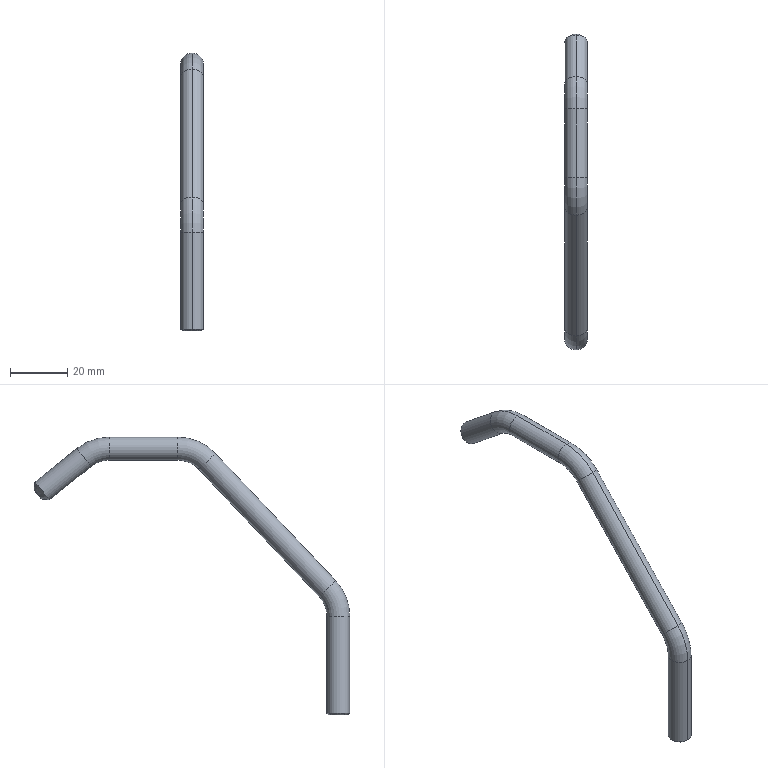Part | STEP file | 8XS234010 | 1 solid | 20 faces | box 8 x 110.249 x 97 mm | volume 8595 mm3 | cylinder 8 | torus 6 | cone 4 | plane 2 | commonest cylinder face diameters 8 x8
STEP:
#1=CARTESIAN_POINT('',(0.,0.,0.));
#2=DIRECTION('',(0.,0.,1.));
#3=DIRECTION('',(1.,0.,0.));
#4=AXIS2_PLACEMENT_3D('',#1,#2,#3);
#5=CARTESIAN_POINT('',(0.,4.,34.438));
#6=VERTEX_POINT('',#5);
#7=CARTESIAN_POINT('',(0.,-4.,34.438));
#8=VERTEX_POINT('',#7);
#9=CARTESIAN_POINT('',(0.,0.,34.438));
#10=DIRECTION('',(0.,0.,1.));
#11=DIRECTION('',(1.,0.,0.));
#12=AXIS2_PLACEMENT_3D('',#9,#10,#11);
#13=CIRCLE('',#12,4.);
#14=CARTESIAN_POINT('',(0.,14.,34.438));
#15=DIRECTION('',(-1.,0.,0.));
#16=DIRECTION('',(0.,0.,1.));
#17=AXIS2_PLACEMENT_3D('',#14,#15,#16);
#18=TOROIDAL_SURFACE('',#17,14.,4.);
#19=CARTESIAN_POINT('',(4.712,4.712));
#20=DIRECTION('',(0.,-1.));
#21=VECTOR('',#20,1.);
#22=LINE('',#19,#21);
#23=(GEOMETRIC_REPRESENTATION_CONTEXT(2)PARAMETRIC_REPRESENTATION_CONTEXT()REPRESENTATION_CONTEXT('',''));
#24=DEFINITIONAL_REPRESENTATION('',(#22),#23);
#25=PCURVE('',#18,#24);
#26=CARTESIAN_POINT('',(0.,0.,34.438));
#27=DIRECTION('',(0.,0.,-1.));
#28=DIRECTION('',(0.,1.,0.));
#29=AXIS2_PLACEMENT_3D('',#26,#27,#28);
#30=CYLINDRICAL_SURFACE('',#29,4.);
#31=CARTESIAN_POINT('',(7.854,0.));
#32=DIRECTION('',(-1.,0.));
#33=VECTOR('',#32,1.);
#34=LINE('',#31,#33);
#35=(GEOMETRIC_REPRESENTATION_CONTEXT(2)PARAMETRIC_REPRESENTATION_CONTEXT()REPRESENTATION_CONTEXT('',''));
#36=DEFINITIONAL_REPRESENTATION('',(#34),#35);
#37=PCURVE('',#30,#36);
#38=SURFACE_CURVE('',#13,(#25,#37),.PCURVE_S1.);
#39=EDGE_CURVE('',#6,#8,#38,.T.);
#40=ORIENTED_EDGE('',*,*,#39,.T.);
#41=CARTESIAN_POINT('',(0.,0.9069,46.79));
#42=VERTEX_POINT('',#41);
#43=CARTESIAN_POINT('',(0.,14.,34.438));
#44=DIRECTION('',(-1.,0.,0.));
#45=DIRECTION('',(0.,0.,1.));
#46=AXIS2_PLACEMENT_3D('',#43,#44,#45);
#47=CIRCLE('',#46,18.);
#48=CARTESIAN_POINT('',(0.,0.));
#49=DIRECTION('',(1.,0.));
#50=VECTOR('',#49,1.);
#51=LINE('',#48,#50);
#52=(GEOMETRIC_REPRESENTATION_CONTEXT(2)PARAMETRIC_REPRESENTATION_CONTEXT()REPRESENTATION_CONTEXT('',''));
#53=DEFINITIONAL_REPRESENTATION('',(#51),#52);
#54=PCURVE('',#18,#53);
#55=CARTESIAN_POINT('',(0.,14.,34.438));
#56=DIRECTION('',(-1.,0.,0.));
#57=DIRECTION('',(0.,0.,1.));
#58=AXIS2_PLACEMENT_3D('',#55,#56,#57);
#59=TOROIDAL_SURFACE('',#58,14.,4.);
#60=CARTESIAN_POINT('',(0.,6.283));
#61=DIRECTION('',(1.,0.));
#62=VECTOR('',#61,1.);
#63=LINE('',#60,#62);
#64=(GEOMETRIC_REPRESENTATION_CONTEXT(2)PARAMETRIC_REPRESENTATION_CONTEXT()REPRESENTATION_CONTEXT('',''));
#65=DEFINITIONAL_REPRESENTATION('',(#63),#64);
#66=PCURVE('',#59,#65);
#67=SURFACE_CURVE('',#47,(#54,#66),.PCURVE_S1.);
#68=EDGE_CURVE('',#8,#42,#67,.T.);
#69=ORIENTED_EDGE('',*,*,#68,.T.);
#70=CARTESIAN_POINT('',(0.,6.726,41.301));
#71=VERTEX_POINT('',#70);
#72=CARTESIAN_POINT('',(0.,3.816,44.045));
#73=DIRECTION('',(0.,0.6862,0.7274));
#74=DIRECTION('',(1.,0.,0.));
#75=AXIS2_PLACEMENT_3D('',#72,#73,#74);
#76=CIRCLE('',#75,4.);
#77=CARTESIAN_POINT('',(5.469,4.712));
#78=DIRECTION('',(0.,-1.));
#79=VECTOR('',#78,1.);
#80=LINE('',#77,#79);
#81=(GEOMETRIC_REPRESENTATION_CONTEXT(2)PARAMETRIC_REPRESENTATION_CONTEXT()REPRESENTATION_CONTEXT('',''));
#82=DEFINITIONAL_REPRESENTATION('',(#80),#81);
#83=PCURVE('',#18,#82);
#84=CARTESIAN_POINT('',(0.,3.816,44.045));
#85=DIRECTION('',(0.,0.6862,0.7274));
#86=DIRECTION('',(0.,-0.7274,0.6862));
#87=AXIS2_PLACEMENT_3D('',#84,#85,#86);
#88=CYLINDRICAL_SURFACE('',#87,4.);
#89=CARTESIAN_POINT('',(1.571,0.));
#90=DIRECTION('',(1.,0.));
#91=VECTOR('',#90,1.);
#92=LINE('',#89,#91);
#93=(GEOMETRIC_REPRESENTATION_CONTEXT(2)PARAMETRIC_REPRESENTATION_CONTEXT()REPRESENTATION_CONTEXT('',''));
#94=DEFINITIONAL_REPRESENTATION('',(#92),#93);
#95=PCURVE('',#88,#94);
#96=SURFACE_CURVE('',#76,(#83,#95),.PCURVE_S1.);
#97=EDGE_CURVE('',#71,#42,#96,.T.);
#98=ORIENTED_EDGE('',*,*,#97,.F.);
#99=CARTESIAN_POINT('',(0.,14.,34.438));
#100=DIRECTION('',(-1.,0.,0.));
#101=DIRECTION('',(0.,0.,1.));
#102=AXIS2_PLACEMENT_3D('',#99,#100,#101);
#103=CIRCLE('',#102,10.);
#104=CARTESIAN_POINT('',(0.,3.142));
#105=DIRECTION('',(1.,0.));
#106=VECTOR('',#105,1.);
#107=LINE('',#104,#106);
#108=(GEOMETRIC_REPRESENTATION_CONTEXT(2)PARAMETRIC_REPRESENTATION_CONTEXT()REPRESENTATION_CONTEXT('',''));
#109=DEFINITIONAL_REPRESENTATION('',(#107),#108);
#110=PCURVE('',#18,#109);
#111=CARTESIAN_POINT('',(0.,3.142));
#112=DIRECTION('',(1.,0.));
#113=VECTOR('',#112,1.);
#114=LINE('',#111,#113);
#115=(GEOMETRIC_REPRESENTATION_CONTEXT(2)PARAMETRIC_REPRESENTATION_CONTEXT()REPRESENTATION_CONTEXT('',''));
#116=DEFINITIONAL_REPRESENTATION('',(#114),#115);
#117=PCURVE('',#59,#116);
#118=SURFACE_CURVE('',#103,(#110,#117),.PCURVE_S1.);
#119=EDGE_CURVE('',#6,#71,#118,.T.);
#120=ORIENTED_EDGE('',*,*,#119,.F.);
#121=EDGE_LOOP('',(#40,#69,#98,#120));
#122=FACE_BOUND('',#121,.T.);
#123=ADVANCED_FACE('',(#122),#18,.T.);
#124=CARTESIAN_POINT('',(0.,48.765,85.862));
#125=VERTEX_POINT('',#124);
#126=CARTESIAN_POINT('',(0.,42.946,91.352));
#127=VERTEX_POINT('',#126);
#128=CARTESIAN_POINT('',(0.,45.856,88.607));
#129=DIRECTION('',(0.,0.6862,0.7274));
#130=DIRECTION('',(1.,0.,0.));
#131=AXIS2_PLACEMENT_3D('',#128,#129,#130);
#132=CIRCLE('',#131,4.);
#133=CARTESIAN_POINT('',(0.,56.039,79.));
#134=DIRECTION('',(-1.,0.,0.));
#135=DIRECTION('',(0.,0.,1.));
#136=AXIS2_PLACEMENT_3D('',#133,#134,#135);
#137=TOROIDAL_SURFACE('',#136,14.,4.);
#138=CARTESIAN_POINT('',(5.469,4.712));
#139=DIRECTION('',(0.,-1.));
#140=VECTOR('',#139,1.);
#141=LINE('',#138,#140);
#142=(GEOMETRIC_REPRESENTATION_CONTEXT(2)PARAMETRIC_REPRESENTATION_CONTEXT()REPRESENTATION_CONTEXT('',''));
#143=DEFINITIONAL_REPRESENTATION('',(#141),#142);
#144=PCURVE('',#137,#143);
#145=CARTESIAN_POINT('',(1.571,61.262));
#146=DIRECTION('',(1.,0.));
#147=VECTOR('',#146,1.);
#148=LINE('',#145,#147);
#149=(GEOMETRIC_REPRESENTATION_CONTEXT(2)PARAMETRIC_REPRESENTATION_CONTEXT()REPRESENTATION_CONTEXT('',''));
#150=DEFINITIONAL_REPRESENTATION('',(#148),#149);
#151=PCURVE('',#88,#150);
#152=SURFACE_CURVE('',#132,(#144,#151),.PCURVE_S1.);
#153=EDGE_CURVE('',#125,#127,#152,.T.);
#154=ORIENTED_EDGE('',*,*,#153,.T.);
#155=CARTESIAN_POINT('',(0.,56.039,97.));
#156=VERTEX_POINT('',#155);
#157=CARTESIAN_POINT('',(0.,56.039,79.));
#158=DIRECTION('',(-1.,0.,0.));
#159=DIRECTION('',(0.,0.,1.));
#160=AXIS2_PLACEMENT_3D('',#157,#158,#159);
#161=CIRCLE('',#160,18.);
#162=CARTESIAN_POINT('',(0.,0.));
#163=DIRECTION('',(1.,0.));
#164=VECTOR('',#163,1.);
#165=LINE('',#162,#164);
#166=(GEOMETRIC_REPRESENTATION_CONTEXT(2)PARAMETRIC_REPRESENTATION_CONTEXT()REPRESENTATION_CONTEXT('',''));
#167=DEFINITIONAL_REPRESENTATION('',(#165),#166);
#168=PCURVE('',#137,#167);
#169=CARTESIAN_POINT('',(0.,56.039,79.));
#170=DIRECTION('',(-1.,0.,0.));
#171=DIRECTION('',(0.,0.,1.));
#172=AXIS2_PLACEMENT_3D('',#169,#170,#171);
#173=TOROIDAL_SURFACE('',#172,14.,4.);
#174=CARTESIAN_POINT('',(0.,6.283));
#175=DIRECTION('',(1.,0.));
#176=VECTOR('',#175,1.);
#177=LINE('',#174,#176);
#178=(GEOMETRIC_REPRESENTATION_CONTEXT(2)PARAMETRIC_REPRESENTATION_CONTEXT()REPRESENTATION_CONTEXT('',''));
#179=DEFINITIONAL_REPRESENTATION('',(#177),#178);
#180=PCURVE('',#173,#179);
#181=SURFACE_CURVE('',#161,(#168,#180),.PCURVE_S1.);
#182=EDGE_CURVE('',#127,#156,#181,.T.);
#183=ORIENTED_EDGE('',*,*,#182,.T.);
#184=CARTESIAN_POINT('',(0.,56.039,89.));
#185=VERTEX_POINT('',#184);
#186=CARTESIAN_POINT('',(0.,56.039,93.));
#187=DIRECTION('',(0.,1.,0.));
#188=DIRECTION('',(1.,0.,0.));
#189=AXIS2_PLACEMENT_3D('',#186,#187,#188);
#190=CIRCLE('',#189,4.);
#191=CARTESIAN_POINT('',(6.283,4.712));
#192=DIRECTION('',(0.,-1.));
#193=VECTOR('',#192,1.);
#194=LINE('',#191,#193);
#195=(GEOMETRIC_REPRESENTATION_CONTEXT(2)PARAMETRIC_REPRESENTATION_CONTEXT()REPRESENTATION_CONTEXT('',''));
#196=DEFINITIONAL_REPRESENTATION('',(#194),#195);
#197=PCURVE('',#137,#196);
#198=CARTESIAN_POINT('',(0.,56.039,93.));
#199=DIRECTION('',(0.,1.,0.));
#200=DIRECTION('',(0.,0.,1.));
#201=AXIS2_PLACEMENT_3D('',#198,#199,#200);
#202=CYLINDRICAL_SURFACE('',#201,4.);
#203=CARTESIAN_POINT('',(1.571,0.));
#204=DIRECTION('',(1.,0.));
#205=VECTOR('',#204,1.);
#206=LINE('',#203,#205);
#207=(GEOMETRIC_REPRESENTATION_CONTEXT(2)PARAMETRIC_REPRESENTATION_CONTEXT()REPRESENTATION_CONTEXT('',''));
#208=DEFINITIONAL_REPRESENTATION('',(#206),#207);
#209=PCURVE('',#202,#208);
#210=SURFACE_CURVE('',#190,(#197,#209),.PCURVE_S1.);
#211=EDGE_CURVE('',#185,#156,#210,.T.);
#212=ORIENTED_EDGE('',*,*,#211,.F.);
#213=CARTESIAN_POINT('',(0.,56.039,79.));
#214=DIRECTION('',(-1.,0.,0.));
#215=DIRECTION('',(0.,0.,1.));
#216=AXIS2_PLACEMENT_3D('',#213,#214,#215);
#217=CIRCLE('',#216,10.);
#218=CARTESIAN_POINT('',(0.,3.142));
#219=DIRECTION('',(1.,0.));
#220=VECTOR('',#219,1.);
#221=LINE('',#218,#220);
#222=(GEOMETRIC_REPRESENTATION_CONTEXT(2)PARAMETRIC_REPRESENTATION_CONTEXT()REPRESENTATION_CONTEXT('',''));
#223=DEFINITIONAL_REPRESENTATION('',(#221),#222);
#224=PCURVE('',#137,#223);
#225=CARTESIAN_POINT('',(0.,3.142));
#226=DIRECTION('',(1.,0.));
#227=VECTOR('',#226,1.);
#228=LINE('',#225,#227);
#229=(GEOMETRIC_REPRESENTATION_CONTEXT(2)PARAMETRIC_REPRESENTATION_CONTEXT()REPRESENTATION_CONTEXT('',''));
#230=DEFINITIONAL_REPRESENTATION('',(#228),#229);
#231=PCURVE('',#173,#230);
#232=SURFACE_CURVE('',#217,(#224,#231),.PCURVE_S1.);
#233=EDGE_CURVE('',#125,#185,#232,.T.);
#234=ORIENTED_EDGE('',*,*,#233,.F.);
#235=EDGE_LOOP('',(#154,#183,#212,#234));
#236=FACE_BOUND('',#235,.T.);
#237=ADVANCED_FACE('',(#236),#137,.T.);
#238=CARTESIAN_POINT('',(0.,80.089,89.));
#239=VERTEX_POINT('',#238);
#240=CARTESIAN_POINT('',(0.,80.089,97.));
#241=VERTEX_POINT('',#240);
#242=CARTESIAN_POINT('',(0.,80.089,93.));
#243=DIRECTION('',(0.,1.,0.));
#244=DIRECTION('',(1.,0.,0.));
#245=AXIS2_PLACEMENT_3D('',#242,#243,#244);
#246=CIRCLE('',#245,4.);
#247=CARTESIAN_POINT('',(0.,80.089,79.));
#248=DIRECTION('',(-1.,0.,0.));
#249=DIRECTION('',(0.,0.,1.));
#250=AXIS2_PLACEMENT_3D('',#247,#248,#249);
#251=TOROIDAL_SURFACE('',#250,14.,4.);
#252=CARTESIAN_POINT('',(0.,4.712));
#253=DIRECTION('',(0.,-1.));
#254=VECTOR('',#253,1.);
#255=LINE('',#252,#254);
#256=(GEOMETRIC_REPRESENTATION_CONTEXT(2)PARAMETRIC_REPRESENTATION_CONTEXT()REPRESENTATION_CONTEXT('',''));
#257=DEFINITIONAL_REPRESENTATION('',(#255),#256);
#258=PCURVE('',#251,#257);
#259=CARTESIAN_POINT('',(1.571,24.05));
#260=DIRECTION('',(1.,0.));
#261=VECTOR('',#260,1.);
#262=LINE('',#259,#261);
#263=(GEOMETRIC_REPRESENTATION_CONTEXT(2)PARAMETRIC_REPRESENTATION_CONTEXT()REPRESENTATION_CONTEXT('',''));
#264=DEFINITIONAL_REPRESENTATION('',(#262),#263);
#265=PCURVE('',#202,#264);
#266=SURFACE_CURVE('',#246,(#258,#265),.PCURVE_S1.);
#267=EDGE_CURVE('',#239,#241,#266,.T.);
#268=ORIENTED_EDGE('',*,*,#267,.T.);
#269=CARTESIAN_POINT('',(0.,91.334,93.056));
#270=VERTEX_POINT('',#269);
#271=CARTESIAN_POINT('',(0.,80.089,79.));
#272=DIRECTION('',(-1.,0.,0.));
#273=DIRECTION('',(0.,0.,1.));
#274=AXIS2_PLACEMENT_3D('',#271,#272,#273);
#275=CIRCLE('',#274,18.);
#276=CARTESIAN_POINT('',(0.,0.));
#277=DIRECTION('',(1.,0.));
#278=VECTOR('',#277,1.);
#279=LINE('',#276,#278);
#280=(GEOMETRIC_REPRESENTATION_CONTEXT(2)PARAMETRIC_REPRESENTATION_CONTEXT()REPRESENTATION_CONTEXT('',''));
#281=DEFINITIONAL_REPRESENTATION('',(#279),#280);
#282=PCURVE('',#251,#281);
#283=CARTESIAN_POINT('',(0.,80.089,79.));
#284=DIRECTION('',(-1.,0.,0.));
#285=DIRECTION('',(0.,0.,1.));
#286=AXIS2_PLACEMENT_3D('',#283,#284,#285);
#287=TOROIDAL_SURFACE('',#286,14.,4.);
#288=CARTESIAN_POINT('',(0.,6.283));
#289=DIRECTION('',(1.,0.));
#290=VECTOR('',#289,1.);
#291=LINE('',#288,#290);
#292=(GEOMETRIC_REPRESENTATION_CONTEXT(2)PARAMETRIC_REPRESENTATION_CONTEXT()REPRESENTATION_CONTEXT('',''));
#293=DEFINITIONAL_REPRESENTATION('',(#291),#292);
#294=PCURVE('',#287,#293);
#295=SURFACE_CURVE('',#275,(#282,#294),.PCURVE_S1.);
#296=EDGE_CURVE('',#241,#270,#295,.T.);
#297=ORIENTED_EDGE('',*,*,#296,.T.);
#298=CARTESIAN_POINT('',(0.,86.336,86.809));
#299=VERTEX_POINT('',#298);
#300=CARTESIAN_POINT('',(0.,88.835,89.932));
#301=DIRECTION('',(0.,0.7809,-0.6247));
#302=DIRECTION('',(1.,0.,0.));
#303=AXIS2_PLACEMENT_3D('',#300,#301,#302);
#304=CIRCLE('',#303,4.);
#305=CARTESIAN_POINT('',(0.6747,4.712));
#306=DIRECTION('',(0.,-1.));
#307=VECTOR('',#306,1.);
#308=LINE('',#305,#307);
#309=(GEOMETRIC_REPRESENTATION_CONTEXT(2)PARAMETRIC_REPRESENTATION_CONTEXT()REPRESENTATION_CONTEXT('',''));
#310=DEFINITIONAL_REPRESENTATION('',(#308),#309);
#311=PCURVE('',#251,#310);
#312=CARTESIAN_POINT('',(0.,88.835,89.932));
#313=DIRECTION('',(0.,0.7809,-0.6247));
#314=DIRECTION('',(0.,0.6247,0.7809));
#315=AXIS2_PLACEMENT_3D('',#312,#313,#314);
#316=CYLINDRICAL_SURFACE('',#315,4.);
#317=CARTESIAN_POINT('',(1.571,0.));
#318=DIRECTION('',(1.,0.));
#319=VECTOR('',#318,1.);
#320=LINE('',#317,#319);
#321=(GEOMETRIC_REPRESENTATION_CONTEXT(2)PARAMETRIC_REPRESENTATION_CONTEXT()REPRESENTATION_CONTEXT('',''));
#322=DEFINITIONAL_REPRESENTATION('',(#320),#321);
#323=PCURVE('',#316,#322);
#324=SURFACE_CURVE('',#304,(#311,#323),.PCURVE_S1.);
#325=EDGE_CURVE('',#299,#270,#324,.T.);
#326=ORIENTED_EDGE('',*,*,#325,.F.);
#327=CARTESIAN_POINT('',(0.,80.089,79.));
#328=DIRECTION('',(-1.,0.,0.));
#329=DIRECTION('',(0.,0.,1.));
#330=AXIS2_PLACEMENT_3D('',#327,#328,#329);
#331=CIRCLE('',#330,10.);
#332=CARTESIAN_POINT('',(0.,3.142));
#333=DIRECTION('',(1.,0.));
#334=VECTOR('',#333,1.);
#335=LINE('',#332,#334);
#336=(GEOMETRIC_REPRESENTATION_CONTEXT(2)PARAMETRIC_REPRESENTATION_CONTEXT()REPRESENTATION_CONTEXT('',''));
#337=DEFINITIONAL_REPRESENTATION('',(#335),#336);
#338=PCURVE('',#251,#337);
#339=CARTESIAN_POINT('',(0.,3.142));
#340=DIRECTION('',(1.,0.));
#341=VECTOR('',#340,1.);
#342=LINE('',#339,#341);
#343=(GEOMETRIC_REPRESENTATION_CONTEXT(2)PARAMETRIC_REPRESENTATION_CONTEXT()REPRESENTATION_CONTEXT('',''));
#344=DEFINITIONAL_REPRESENTATION('',(#342),#343);
#345=PCURVE('',#287,#344);
#346=SURFACE_CURVE('',#331,(#338,#345),.PCURVE_S1.);
#347=EDGE_CURVE('',#239,#299,#346,.T.);
#348=ORIENTED_EDGE('',*,*,#347,.F.);
#349=EDGE_LOOP('',(#268,#297,#326,#348));
#350=FACE_BOUND('',#349,.T.);
#351=ADVANCED_FACE('',(#350),#251,.T.);
#352=CARTESIAN_POINT('',(0.,106.249,78.562));
#353=VERTEX_POINT('',#352);
#354=CARTESIAN_POINT('',(0.,103.751,75.438));
#355=VERTEX_POINT('',#354);
#356=CARTESIAN_POINT('',(0.,105.,77.));
#357=DIRECTION('',(0.,0.7809,-0.6247));
#358=DIRECTION('',(0.,0.6247,0.7809));
#359=AXIS2_PLACEMENT_3D('',#356,#357,#358);
#360=CIRCLE('',#359,2.);
#361=CARTESIAN_POINT('',(0.,105.,77.));
#362=DIRECTION('',(0.,-0.7809,0.6247));
#363=DIRECTION('',(0.,-0.6247,-0.7809));
#364=AXIS2_PLACEMENT_3D('',#361,#362,#363);
#365=CONICAL_SURFACE('',#364,2.,0.7854);
#366=CARTESIAN_POINT('',(3.142,0.));
#367=DIRECTION('',(-1.,0.));
#368=VECTOR('',#367,1.);
#369=LINE('',#366,#368);
#370=(GEOMETRIC_REPRESENTATION_CONTEXT(2)PARAMETRIC_REPRESENTATION_CONTEXT()REPRESENTATION_CONTEXT('',''));
#371=DEFINITIONAL_REPRESENTATION('',(#369),#370);
#372=PCURVE('',#365,#371);
#373=CARTESIAN_POINT('',(0.,105.,77.));
#374=DIRECTION('',(0.,0.7809,-0.6247));
#375=DIRECTION('',(1.,0.,0.));
#376=AXIS2_PLACEMENT_3D('',#373,#374,#375);
#377=PLANE('',#376);
#378=CARTESIAN_POINT('',(0.,0.));
#379=DIRECTION('',(0.,-1.));
#380=AXIS2_PLACEMENT_2D('',#378,#379);
#381=CIRCLE('',#380,2.);
#382=(GEOMETRIC_REPRESENTATION_CONTEXT(2)PARAMETRIC_REPRESENTATION_CONTEXT()REPRESENTATION_CONTEXT('',''));
#383=DEFINITIONAL_REPRESENTATION('',(#381),#382);
#384=PCURVE('',#377,#383);
#385=SURFACE_CURVE('',#360,(#372,#384),.PCURVE_S1.);
#386=EDGE_CURVE('',#353,#355,#385,.T.);
#387=ORIENTED_EDGE('',*,*,#386,.F.);
#388=CARTESIAN_POINT('',(0.,105.937,81.373));
#389=VERTEX_POINT('',#388);
#390=CARTESIAN_POINT('',(0.,106.249,78.562));
#391=DIRECTION('',(0.,-0.1104,0.9939));
#392=VECTOR('',#391,1.);
#393=LINE('',#390,#392);
#394=CARTESIAN_POINT('',(3.142,0.));
#395=DIRECTION('',(0.,1.));
#396=VECTOR('',#395,1.);
#397=LINE('',#394,#396);
#398=(GEOMETRIC_REPRESENTATION_CONTEXT(2)PARAMETRIC_REPRESENTATION_CONTEXT()REPRESENTATION_CONTEXT('',''));
#399=DEFINITIONAL_REPRESENTATION('',(#397),#398);
#400=PCURVE('',#365,#399);
#401=CARTESIAN_POINT('',(0.,105.,77.));
#402=DIRECTION('',(0.,-0.7809,0.6247));
#403=DIRECTION('',(0.,-0.6247,-0.7809));
#404=AXIS2_PLACEMENT_3D('',#401,#402,#403);
#405=CONICAL_SURFACE('',#404,2.,0.7854);
#406=CARTESIAN_POINT('',(3.142,0.));
#407=DIRECTION('',(0.,1.));
#408=VECTOR('',#407,1.);
#409=LINE('',#406,#408);
#410=(GEOMETRIC_REPRESENTATION_CONTEXT(2)PARAMETRIC_REPRESENTATION_CONTEXT()REPRESENTATION_CONTEXT('',''));
#411=DEFINITIONAL_REPRESENTATION('',(#409),#410);
#412=PCURVE('',#405,#411);
#413=SURFACE_CURVE('',#393,(#400,#412),.PCURVE_S1.);
#414=EDGE_CURVE('',#353,#389,#413,.T.);
#415=ORIENTED_EDGE('',*,*,#414,.T.);
#416=CARTESIAN_POINT('',(0.,100.939,75.126));
#417=VERTEX_POINT('',#416);
#418=CARTESIAN_POINT('',(0.,103.438,78.249));
#419=DIRECTION('',(0.,-0.7809,0.6247));
#420=DIRECTION('',(0.,0.6247,0.7809));
#421=AXIS2_PLACEMENT_3D('',#418,#419,#420);
#422=CIRCLE('',#421,4.);
#423=CARTESIAN_POINT('',(-3.142,2.));
#424=DIRECTION('',(1.,0.));
#425=VECTOR('',#424,1.);
#426=LINE('',#423,#425);
#427=(GEOMETRIC_REPRESENTATION_CONTEXT(2)PARAMETRIC_REPRESENTATION_CONTEXT()REPRESENTATION_CONTEXT('',''));
#428=DEFINITIONAL_REPRESENTATION('',(#426),#427);
#429=PCURVE('',#365,#428);
#430=CARTESIAN_POINT('',(0.,88.835,89.932));
#431=DIRECTION('',(0.,0.7809,-0.6247));
#432=DIRECTION('',(0.,0.6247,0.7809));
#433=AXIS2_PLACEMENT_3D('',#430,#431,#432);
#434=CYLINDRICAL_SURFACE('',#433,4.);
#435=CARTESIAN_POINT('',(6.283,18.702));
#436=DIRECTION('',(-1.,0.));
#437=VECTOR('',#436,1.);
#438=LINE('',#435,#437);
#439=(GEOMETRIC_REPRESENTATION_CONTEXT(2)PARAMETRIC_REPRESENTATION_CONTEXT()REPRESENTATION_CONTEXT('',''));
#440=DEFINITIONAL_REPRESENTATION('',(#438),#439);
#441=PCURVE('',#434,#440);
#442=SURFACE_CURVE('',#422,(#429,#441),.PCURVE_S1.);
#443=EDGE_CURVE('',#417,#389,#442,.T.);
#444=ORIENTED_EDGE('',*,*,#443,.F.);
#445=CARTESIAN_POINT('',(0.,103.751,75.438));
#446=DIRECTION('',(0.,-0.9939,-0.1104));
#447=VECTOR('',#446,1.);
#448=LINE('',#445,#447);
#449=CARTESIAN_POINT('',(0.,0.));
#450=DIRECTION('',(0.,1.));
#451=VECTOR('',#450,1.);
#452=LINE('',#449,#451);
#453=(GEOMETRIC_REPRESENTATION_CONTEXT(2)PARAMETRIC_REPRESENTATION_CONTEXT()REPRESENTATION_CONTEXT('',''));
#454=DEFINITIONAL_REPRESENTATION('',(#452),#453);
#455=PCURVE('',#365,#454);
#456=CARTESIAN_POINT('',(6.283,0.));
#457=DIRECTION('',(0.,1.));
#458=VECTOR('',#457,1.);
#459=LINE('',#456,#458);
#460=(GEOMETRIC_REPRESENTATION_CONTEXT(2)PARAMETRIC_REPRESENTATION_CONTEXT()REPRESENTATION_CONTEXT('',''));
#461=DEFINITIONAL_REPRESENTATION('',(#459),#460);
#462=PCURVE('',#405,#461);
#463=SURFACE_CURVE('',#448,(#455,#462),.PCURVE_S1.);
#464=EDGE_CURVE('',#355,#417,#463,.T.);
#465=ORIENTED_EDGE('',*,*,#464,.F.);
#466=EDGE_LOOP('',(#387,#415,#444,#465));
#467=FACE_BOUND('',#466,.T.);
#468=ADVANCED_FACE('',(#467),#365,.T.);
#469=CARTESIAN_POINT('',(0.,3.5,0.));
#470=VERTEX_POINT('',#469);
#471=CARTESIAN_POINT('',(0.,-3.5,0.));
#472=VERTEX_POINT('',#471);
#473=CARTESIAN_POINT('',(0.,0.,0.));
#474=DIRECTION('',(0.,0.,-1.));
#475=DIRECTION('',(1.,0.,0.));
#476=AXIS2_PLACEMENT_3D('',#473,#474,#475);
#477=CIRCLE('',#476,3.5);
#478=CARTESIAN_POINT('',(0.,0.,0.5));
#479=DIRECTION('',(0.,0.,1.));
#480=DIRECTION('',(0.,-1.,0.));
#481=AXIS2_PLACEMENT_3D('',#478,#479,#480);
#482=CONICAL_SURFACE('',#481,4.,0.7854);
#483=CARTESIAN_POINT('',(7.854,-0.5));
#484=DIRECTION('',(-1.,0.));
#485=VECTOR('',#484,1.);
#486=LINE('',#483,#485);
#487=(GEOMETRIC_REPRESENTATION_CONTEXT(2)PARAMETRIC_REPRESENTATION_CONTEXT()REPRESENTATION_CONTEXT('',''));
#488=DEFINITIONAL_REPRESENTATION('',(#486),#487);
#489=PCURVE('',#482,#488);
#490=CARTESIAN_POINT('',(0.,0.,0.));
#491=DIRECTION('',(0.,0.,1.));
#492=DIRECTION('',(1.,0.,0.));
#493=AXIS2_PLACEMENT_3D('',#490,#491,#492);
#494=PLANE('',#493);
#495=CARTESIAN_POINT('',(3.5,0.));
#496=CARTESIAN_POINT('',(3.5,-6.062));
#497=CARTESIAN_POINT('',(-1.75,-3.031));
#498=CARTESIAN_POINT('',(-7.,0.));
#499=CARTESIAN_POINT('',(-1.75,3.031));
#500=CARTESIAN_POINT('',(3.5,6.062));
#501=CARTESIAN_POINT('',(3.5,0.));
#502=(BOUNDED_CURVE()B_SPLINE_CURVE(2,(#495,#496,#497,#498,#499,#500,#501),.UNSPECIFIED.,.T.,.F.)B_SPLINE_CURVE_WITH_KNOTS((1,2,2,2,2,1),(-2.094,0.,2.094,4.189,6.283,8.378),.UNSPECIFIED.)CURVE()GEOMETRIC_REPRESENTATION_ITEM()RATIONAL_B_SPLINE_CURVE((1.,0.5,1.,0.5,1.,0.5,1.))REPRESENTATION_ITEM(''));
#503=(GEOMETRIC_REPRESENTATION_CONTEXT(2)PARAMETRIC_REPRESENTATION_CONTEXT()REPRESENTATION_CONTEXT('',''));
#504=DEFINITIONAL_REPRESENTATION('',(#502),#503);
#505=PCURVE('',#494,#504);
#506=SURFACE_CURVE('',#477,(#489,#505),.PCURVE_S1.);
#507=EDGE_CURVE('',#470,#472,#506,.T.);
#508=ORIENTED_EDGE('',*,*,#507,.F.);
#509=CARTESIAN_POINT('',(0.,4.,0.5));
#510=VERTEX_POINT('',#509);
#511=CARTESIAN_POINT('',(0.,4.,0.5));
#512=DIRECTION('',(0.,0.7071,0.7071));
#513=VECTOR('',#512,1.);
#514=LINE('',#511,#513);
#515=CARTESIAN_POINT('',(3.142,0.));
#516=DIRECTION('',(0.,1.));
#517=VECTOR('',#516,1.);
#518=LINE('',#515,#517);
#519=(GEOMETRIC_REPRESENTATION_CONTEXT(2)PARAMETRIC_REPRESENTATION_CONTEXT()REPRESENTATION_CONTEXT('',''));
#520=DEFINITIONAL_REPRESENTATION('',(#518),#519);
#521=PCURVE('',#482,#520);
#522=CARTESIAN_POINT('',(0.,0.,0.5));
#523=DIRECTION('',(0.,0.,1.));
#524=DIRECTION('',(0.,-1.,0.));
#525=AXIS2_PLACEMENT_3D('',#522,#523,#524);
#526=CONICAL_SURFACE('',#525,4.,0.7854);
#527=CARTESIAN_POINT('',(3.142,0.));
#528=DIRECTION('',(0.,1.));
#529=VECTOR('',#528,1.);
#530=LINE('',#527,#529);
#531=(GEOMETRIC_REPRESENTATION_CONTEXT(2)PARAMETRIC_REPRESENTATION_CONTEXT()REPRESENTATION_CONTEXT('',''));
#532=DEFINITIONAL_REPRESENTATION('',(#530),#531);
#533=PCURVE('',#526,#532);
#534=SURFACE_CURVE('',#514,(#521,#533),.PCURVE_S1.);
#535=EDGE_CURVE('',#470,#510,#534,.T.);
#536=ORIENTED_EDGE('',*,*,#535,.T.);
#537=CARTESIAN_POINT('',(0.,-4.,0.5));
#538=VERTEX_POINT('',#537);
#539=CARTESIAN_POINT('',(0.,0.,0.5));
#540=DIRECTION('',(0.,0.,1.));
#541=DIRECTION('',(0.,-1.,0.));
#542=AXIS2_PLACEMENT_3D('',#539,#540,#541);
#543=CIRCLE('',#542,4.);
#544=CARTESIAN_POINT('',(0.,0.));
#545=DIRECTION('',(1.,0.));
#546=VECTOR('',#545,1.);
#547=LINE('',#544,#546);
#548=(GEOMETRIC_REPRESENTATION_CONTEXT(2)PARAMETRIC_REPRESENTATION_CONTEXT()REPRESENTATION_CONTEXT('',''));
#549=DEFINITIONAL_REPRESENTATION('',(#547),#548);
#550=PCURVE('',#482,#549);
#551=CARTESIAN_POINT('',(0.,0.,34.438));
#552=DIRECTION('',(0.,0.,-1.));
#553=DIRECTION('',(0.,1.,0.));
#554=AXIS2_PLACEMENT_3D('',#551,#552,#553);
#555=CYLINDRICAL_SURFACE('',#554,4.);
#556=CARTESIAN_POINT('',(3.142,33.938));
#557=DIRECTION('',(-1.,0.));
#558=VECTOR('',#557,1.);
#559=LINE('',#556,#558);
#560=(GEOMETRIC_REPRESENTATION_CONTEXT(2)PARAMETRIC_REPRESENTATION_CONTEXT()REPRESENTATION_CONTEXT('',''));
#561=DEFINITIONAL_REPRESENTATION('',(#559),#560);
#562=PCURVE('',#555,#561);
#563=SURFACE_CURVE('',#543,(#550,#562),.PCURVE_S1.);
#564=EDGE_CURVE('',#538,#510,#563,.T.);
#565=ORIENTED_EDGE('',*,*,#564,.F.);
#566=CARTESIAN_POINT('',(0.,-4.,0.5));
#567=DIRECTION('',(0.,-0.7071,0.7071));
#568=VECTOR('',#567,1.);
#569=LINE('',#566,#568);
#570=CARTESIAN_POINT('',(0.,0.));
#571=DIRECTION('',(0.,1.));
#572=VECTOR('',#571,1.);
#573=LINE('',#570,#572);
#574=(GEOMETRIC_REPRESENTATION_CONTEXT(2)PARAMETRIC_REPRESENTATION_CONTEXT()REPRESENTATION_CONTEXT('',''));
#575=DEFINITIONAL_REPRESENTATION('',(#573),#574);
#576=PCURVE('',#482,#575);
#577=CARTESIAN_POINT('',(6.283,0.));
#578=DIRECTION('',(0.,1.));
#579=VECTOR('',#578,1.);
#580=LINE('',#577,#579);
#581=(GEOMETRIC_REPRESENTATION_CONTEXT(2)PARAMETRIC_REPRESENTATION_CONTEXT()REPRESENTATION_CONTEXT('',''));
#582=DEFINITIONAL_REPRESENTATION('',(#580),#581);
#583=PCURVE('',#526,#582);
#584=SURFACE_CURVE('',#569,(#576,#583),.PCURVE_S1.);
#585=EDGE_CURVE('',#472,#538,#584,.T.);
#586=ORIENTED_EDGE('',*,*,#585,.F.);
#587=EDGE_LOOP('',(#508,#536,#565,#586));
#588=FACE_BOUND('',#587,.T.);
#589=ADVANCED_FACE('',(#588),#482,.T.);
#590=CARTESIAN_POINT('',(0.,0.,34.438));
#591=DIRECTION('',(0.,0.,1.));
#592=DIRECTION('',(1.,0.,0.));
#593=AXIS2_PLACEMENT_3D('',#590,#591,#592);
#594=CIRCLE('',#593,4.);
#595=CARTESIAN_POINT('',(7.854,0.));
#596=DIRECTION('',(-1.,0.));
#597=VECTOR('',#596,1.);
#598=LINE('',#595,#597);
#599=(GEOMETRIC_REPRESENTATION_CONTEXT(2)PARAMETRIC_REPRESENTATION_CONTEXT()REPRESENTATION_CONTEXT('',''));
#600=DEFINITIONAL_REPRESENTATION('',(#598),#599);
#601=PCURVE('',#555,#600);
#602=CARTESIAN_POINT('',(4.712,10.996));
#603=DIRECTION('',(0.,-1.));
#604=VECTOR('',#603,1.);
#605=LINE('',#602,#604);
#606=(GEOMETRIC_REPRESENTATION_CONTEXT(2)PARAMETRIC_REPRESENTATION_CONTEXT()REPRESENTATION_CONTEXT('',''));
#607=DEFINITIONAL_REPRESENTATION('',(#605),#606);
#608=PCURVE('',#59,#607);
#609=SURFACE_CURVE('',#594,(#601,#608),.PCURVE_S1.);
#610=EDGE_CURVE('',#8,#6,#609,.T.);
#611=ORIENTED_EDGE('',*,*,#610,.F.);
#612=CARTESIAN_POINT('',(0.,-4.,34.438));
#613=DIRECTION('',(0.,0.,-1.));
#614=VECTOR('',#613,1.);
#615=LINE('',#612,#614);
#616=CARTESIAN_POINT('',(3.142,0.));
#617=DIRECTION('',(0.,1.));
#618=VECTOR('',#617,1.);
#619=LINE('',#616,#618);
#620=(GEOMETRIC_REPRESENTATION_CONTEXT(2)PARAMETRIC_REPRESENTATION_CONTEXT()REPRESENTATION_CONTEXT('',''));
#621=DEFINITIONAL_REPRESENTATION('',(#619),#620);
#622=PCURVE('',#555,#621);
#623=CARTESIAN_POINT('',(3.142,0.));
#624=DIRECTION('',(0.,1.));
#625=VECTOR('',#624,1.);
#626=LINE('',#623,#625);
#627=(GEOMETRIC_REPRESENTATION_CONTEXT(2)PARAMETRIC_REPRESENTATION_CONTEXT()REPRESENTATION_CONTEXT('',''));
#628=DEFINITIONAL_REPRESENTATION('',(#626),#627);
#629=PCURVE('',#30,#628);
#630=SURFACE_CURVE('',#615,(#622,#629),.PCURVE_S1.);
#631=EDGE_CURVE('',#8,#538,#630,.T.);
#632=ORIENTED_EDGE('',*,*,#631,.T.);
#633=ORIENTED_EDGE('',*,*,#564,.T.);
#634=CARTESIAN_POINT('',(0.,4.,34.438));
#635=DIRECTION('',(0.,0.,-1.));
#636=VECTOR('',#635,1.);
#637=LINE('',#634,#636);
#638=CARTESIAN_POINT('',(0.,0.));
#639=DIRECTION('',(0.,1.));
#640=VECTOR('',#639,1.);
#641=LINE('',#638,#640);
#642=(GEOMETRIC_REPRESENTATION_CONTEXT(2)PARAMETRIC_REPRESENTATION_CONTEXT()REPRESENTATION_CONTEXT('',''));
#643=DEFINITIONAL_REPRESENTATION('',(#641),#642);
#644=PCURVE('',#555,#643);
#645=CARTESIAN_POINT('',(6.283,0.));
#646=DIRECTION('',(0.,1.));
#647=VECTOR('',#646,1.);
#648=LINE('',#645,#647);
#649=(GEOMETRIC_REPRESENTATION_CONTEXT(2)PARAMETRIC_REPRESENTATION_CONTEXT()REPRESENTATION_CONTEXT('',''));
#650=DEFINITIONAL_REPRESENTATION('',(#648),#649);
#651=PCURVE('',#30,#650);
#652=SURFACE_CURVE('',#637,(#644,#651),.PCURVE_S1.);
#653=EDGE_CURVE('',#6,#510,#652,.T.);
#654=ORIENTED_EDGE('',*,*,#653,.F.);
#655=EDGE_LOOP('',(#611,#632,#633,#654));
#656=FACE_BOUND('',#655,.T.);
#657=ADVANCED_FACE('',(#656),#555,.T.);
#658=CARTESIAN_POINT('',(0.,3.816,44.045));
#659=DIRECTION('',(0.,0.6862,0.7274));
#660=DIRECTION('',(1.,0.,0.));
#661=AXIS2_PLACEMENT_3D('',#658,#659,#660);
#662=CIRCLE('',#661,4.);
#663=CARTESIAN_POINT('',(0.,3.816,44.045));
#664=DIRECTION('',(0.,0.6862,0.7274));
#665=DIRECTION('',(0.,-0.7274,0.6862));
#666=AXIS2_PLACEMENT_3D('',#663,#664,#665);
#667=CYLINDRICAL_SURFACE('',#666,4.);
#668=CARTESIAN_POINT('',(-4.712,0.));
#669=DIRECTION('',(1.,0.));
#670=VECTOR('',#669,1.);
#671=LINE('',#668,#670);
#672=(GEOMETRIC_REPRESENTATION_CONTEXT(2)PARAMETRIC_REPRESENTATION_CONTEXT()REPRESENTATION_CONTEXT('',''));
#673=DEFINITIONAL_REPRESENTATION('',(#671),#672);
#674=PCURVE('',#667,#673);
#675=CARTESIAN_POINT('',(5.469,10.996));
#676=DIRECTION('',(0.,-1.));
#677=VECTOR('',#676,1.);
#678=LINE('',#675,#677);
#679=(GEOMETRIC_REPRESENTATION_CONTEXT(2)PARAMETRIC_REPRESENTATION_CONTEXT()REPRESENTATION_CONTEXT('',''));
#680=DEFINITIONAL_REPRESENTATION('',(#678),#679);
#681=PCURVE('',#59,#680);
#682=SURFACE_CURVE('',#662,(#674,#681),.PCURVE_S1.);
#683=EDGE_CURVE('',#42,#71,#682,.T.);
#684=ORIENTED_EDGE('',*,*,#683,.T.);
#685=CARTESIAN_POINT('',(0.,6.726,41.301));
#686=DIRECTION('',(0.,0.6862,0.7274));
#687=VECTOR('',#686,1.);
#688=LINE('',#685,#687);
#689=CARTESIAN_POINT('',(3.142,0.));
#690=DIRECTION('',(0.,1.));
#691=VECTOR('',#690,1.);
#692=LINE('',#689,#691);
#693=(GEOMETRIC_REPRESENTATION_CONTEXT(2)PARAMETRIC_REPRESENTATION_CONTEXT()REPRESENTATION_CONTEXT('',''));
#694=DEFINITIONAL_REPRESENTATION('',(#692),#693);
#695=PCURVE('',#667,#694);
#696=CARTESIAN_POINT('',(3.142,0.));
#697=DIRECTION('',(0.,1.));
#698=VECTOR('',#697,1.);
#699=LINE('',#696,#698);
#700=(GEOMETRIC_REPRESENTATION_CONTEXT(2)PARAMETRIC_REPRESENTATION_CONTEXT()REPRESENTATION_CONTEXT('',''));
#701=DEFINITIONAL_REPRESENTATION('',(#699),#700);
#702=PCURVE('',#88,#701);
#703=SURFACE_CURVE('',#688,(#695,#702),.PCURVE_S1.);
#704=EDGE_CURVE('',#71,#125,#703,.T.);
#705=ORIENTED_EDGE('',*,*,#704,.T.);
#706=CARTESIAN_POINT('',(0.,45.856,88.607));
#707=DIRECTION('',(0.,0.6862,0.7274));
#708=DIRECTION('',(1.,0.,0.));
#709=AXIS2_PLACEMENT_3D('',#706,#707,#708);
#710=CIRCLE('',#709,4.);
#711=CARTESIAN_POINT('',(-4.712,61.262));
#712=DIRECTION('',(1.,0.));
#713=VECTOR('',#712,1.);
#714=LINE('',#711,#713);
#715=(GEOMETRIC_REPRESENTATION_CONTEXT(2)PARAMETRIC_REPRESENTATION_CONTEXT()REPRESENTATION_CONTEXT('',''));
#716=DEFINITIONAL_REPRESENTATION('',(#714),#715);
#717=PCURVE('',#667,#716);
#718=CARTESIAN_POINT('',(5.469,10.996));
#719=DIRECTION('',(0.,-1.));
#720=VECTOR('',#719,1.);
#721=LINE('',#718,#720);
#722=(GEOMETRIC_REPRESENTATION_CONTEXT(2)PARAMETRIC_REPRESENTATION_CONTEXT()REPRESENTATION_CONTEXT('',''));
#723=DEFINITIONAL_REPRESENTATION('',(#721),#722);
#724=PCURVE('',#173,#723);
#725=SURFACE_CURVE('',#710,(#717,#724),.PCURVE_S1.);
#726=EDGE_CURVE('',#127,#125,#725,.T.);
#727=ORIENTED_EDGE('',*,*,#726,.F.);
#728=CARTESIAN_POINT('',(0.,0.9069,46.79));
#729=DIRECTION('',(0.,0.6862,0.7274));
#730=VECTOR('',#729,1.);
#731=LINE('',#728,#730);
#732=CARTESIAN_POINT('',(0.,0.));
#733=DIRECTION('',(0.,1.));
#734=VECTOR('',#733,1.);
#735=LINE('',#732,#734);
#736=(GEOMETRIC_REPRESENTATION_CONTEXT(2)PARAMETRIC_REPRESENTATION_CONTEXT()REPRESENTATION_CONTEXT('',''));
#737=DEFINITIONAL_REPRESENTATION('',(#735),#736);
#738=PCURVE('',#667,#737);
#739=CARTESIAN_POINT('',(6.283,0.));
#740=DIRECTION('',(0.,1.));
#741=VECTOR('',#740,1.);
#742=LINE('',#739,#741);
#743=(GEOMETRIC_REPRESENTATION_CONTEXT(2)PARAMETRIC_REPRESENTATION_CONTEXT()REPRESENTATION_CONTEXT('',''));
#744=DEFINITIONAL_REPRESENTATION('',(#742),#743);
#745=PCURVE('',#88,#744);
#746=SURFACE_CURVE('',#731,(#738,#745),.PCURVE_S1.);
#747=EDGE_CURVE('',#42,#127,#746,.T.);
#748=ORIENTED_EDGE('',*,*,#747,.F.);
#749=EDGE_LOOP('',(#684,#705,#727,#748));
#750=FACE_BOUND('',#749,.T.);
#751=ADVANCED_FACE('',(#750),#667,.T.);
#752=CARTESIAN_POINT('',(0.,56.039,93.));
#753=DIRECTION('',(0.,1.,0.));
#754=DIRECTION('',(1.,0.,0.));
#755=AXIS2_PLACEMENT_3D('',#752,#753,#754);
#756=CIRCLE('',#755,4.);
#757=CARTESIAN_POINT('',(0.,56.039,93.));
#758=DIRECTION('',(0.,1.,0.));
#759=DIRECTION('',(0.,0.,1.));
#760=AXIS2_PLACEMENT_3D('',#757,#758,#759);
#761=CYLINDRICAL_SURFACE('',#760,4.);
#762=CARTESIAN_POINT('',(-4.712,0.));
#763=DIRECTION('',(1.,0.));
#764=VECTOR('',#763,1.);
#765=LINE('',#762,#764);
#766=(GEOMETRIC_REPRESENTATION_CONTEXT(2)PARAMETRIC_REPRESENTATION_CONTEXT()REPRESENTATION_CONTEXT('',''));
#767=DEFINITIONAL_REPRESENTATION('',(#765),#766);
#768=PCURVE('',#761,#767);
#769=CARTESIAN_POINT('',(6.283,10.996));
#770=DIRECTION('',(0.,-1.));
#771=VECTOR('',#770,1.);
#772=LINE('',#769,#771);
#773=(GEOMETRIC_REPRESENTATION_CONTEXT(2)PARAMETRIC_REPRESENTATION_CONTEXT()REPRESENTATION_CONTEXT('',''));
#774=DEFINITIONAL_REPRESENTATION('',(#772),#773);
#775=PCURVE('',#173,#774);
#776=SURFACE_CURVE('',#756,(#768,#775),.PCURVE_S1.);
#777=EDGE_CURVE('',#156,#185,#776,.T.);
#778=ORIENTED_EDGE('',*,*,#777,.T.);
#779=CARTESIAN_POINT('',(0.,56.039,89.));
#780=DIRECTION('',(0.,1.,0.));
#781=VECTOR('',#780,1.);
#782=LINE('',#779,#781);
#783=CARTESIAN_POINT('',(3.142,0.));
#784=DIRECTION('',(0.,1.));
#785=VECTOR('',#784,1.);
#786=LINE('',#783,#785);
#787=(GEOMETRIC_REPRESENTATION_CONTEXT(2)PARAMETRIC_REPRESENTATION_CONTEXT()REPRESENTATION_CONTEXT('',''));
#788=DEFINITIONAL_REPRESENTATION('',(#786),#787);
#789=PCURVE('',#761,#788);
#790=CARTESIAN_POINT('',(3.142,0.));
#791=DIRECTION('',(0.,1.));
#792=VECTOR('',#791,1.);
#793=LINE('',#790,#792);
#794=(GEOMETRIC_REPRESENTATION_CONTEXT(2)PARAMETRIC_REPRESENTATION_CONTEXT()REPRESENTATION_CONTEXT('',''));
#795=DEFINITIONAL_REPRESENTATION('',(#793),#794);
#796=PCURVE('',#202,#795);
#797=SURFACE_CURVE('',#782,(#789,#796),.PCURVE_S1.);
#798=EDGE_CURVE('',#185,#239,#797,.T.);
#799=ORIENTED_EDGE('',*,*,#798,.T.);
#800=CARTESIAN_POINT('',(0.,80.089,93.));
#801=DIRECTION('',(0.,1.,0.));
#802=DIRECTION('',(1.,0.,0.));
#803=AXIS2_PLACEMENT_3D('',#800,#801,#802);
#804=CIRCLE('',#803,4.);
#805=CARTESIAN_POINT('',(-4.712,24.05));
#806=DIRECTION('',(1.,0.));
#807=VECTOR('',#806,1.);
#808=LINE('',#805,#807);
#809=(GEOMETRIC_REPRESENTATION_CONTEXT(2)PARAMETRIC_REPRESENTATION_CONTEXT()REPRESENTATION_CONTEXT('',''));
#810=DEFINITIONAL_REPRESENTATION('',(#808),#809);
#811=PCURVE('',#761,#810);
#812=CARTESIAN_POINT('',(0.,10.996));
#813=DIRECTION('',(0.,-1.));
#814=VECTOR('',#813,1.);
#815=LINE('',#812,#814);
#816=(GEOMETRIC_REPRESENTATION_CONTEXT(2)PARAMETRIC_REPRESENTATION_CONTEXT()REPRESENTATION_CONTEXT('',''));
#817=DEFINITIONAL_REPRESENTATION('',(#815),#816);
#818=PCURVE('',#287,#817);
#819=SURFACE_CURVE('',#804,(#811,#818),.PCURVE_S1.);
#820=EDGE_CURVE('',#241,#239,#819,.T.);
#821=ORIENTED_EDGE('',*,*,#820,.F.);
#822=CARTESIAN_POINT('',(0.,56.039,97.));
#823=DIRECTION('',(0.,1.,0.));
#824=VECTOR('',#823,1.);
#825=LINE('',#822,#824);
#826=CARTESIAN_POINT('',(0.,0.));
#827=DIRECTION('',(0.,1.));
#828=VECTOR('',#827,1.);
#829=LINE('',#826,#828);
#830=(GEOMETRIC_REPRESENTATION_CONTEXT(2)PARAMETRIC_REPRESENTATION_CONTEXT()REPRESENTATION_CONTEXT('',''));
#831=DEFINITIONAL_REPRESENTATION('',(#829),#830);
#832=PCURVE('',#761,#831);
#833=CARTESIAN_POINT('',(6.283,0.));
#834=DIRECTION('',(0.,1.));
#835=VECTOR('',#834,1.);
#836=LINE('',#833,#835);
#837=(GEOMETRIC_REPRESENTATION_CONTEXT(2)PARAMETRIC_REPRESENTATION_CONTEXT()REPRESENTATION_CONTEXT('',''));
#838=DEFINITIONAL_REPRESENTATION('',(#836),#837);
#839=PCURVE('',#202,#838);
#840=SURFACE_CURVE('',#825,(#832,#839),.PCURVE_S1.);
#841=EDGE_CURVE('',#156,#241,#840,.T.);
#842=ORIENTED_EDGE('',*,*,#841,.F.);
#843=EDGE_LOOP('',(#778,#799,#821,#842));
#844=FACE_BOUND('',#843,.T.);
#845=ADVANCED_FACE('',(#844),#761,.T.);
#846=CARTESIAN_POINT('',(0.,88.835,89.932));
#847=DIRECTION('',(0.,0.7809,-0.6247));
#848=DIRECTION('',(1.,0.,0.));
#849=AXIS2_PLACEMENT_3D('',#846,#847,#848);
#850=CIRCLE('',#849,4.);
#851=CARTESIAN_POINT('',(-4.712,0.));
#852=DIRECTION('',(1.,0.));
#853=VECTOR('',#852,1.);
#854=LINE('',#851,#853);
#855=(GEOMETRIC_REPRESENTATION_CONTEXT(2)PARAMETRIC_REPRESENTATION_CONTEXT()REPRESENTATION_CONTEXT('',''));
#856=DEFINITIONAL_REPRESENTATION('',(#854),#855);
#857=PCURVE('',#434,#856);
#858=CARTESIAN_POINT('',(0.6747,10.996));
#859=DIRECTION('',(0.,-1.));
#860=VECTOR('',#859,1.);
#861=LINE('',#858,#860);
#862=(GEOMETRIC_REPRESENTATION_CONTEXT(2)PARAMETRIC_REPRESENTATION_CONTEXT()REPRESENTATION_CONTEXT('',''));
#863=DEFINITIONAL_REPRESENTATION('',(#861),#862);
#864=PCURVE('',#287,#863);
#865=SURFACE_CURVE('',#850,(#857,#864),.PCURVE_S1.);
#866=EDGE_CURVE('',#270,#299,#865,.T.);
#867=ORIENTED_EDGE('',*,*,#866,.T.);
#868=CARTESIAN_POINT('',(0.,86.336,86.809));
#869=DIRECTION('',(0.,0.7809,-0.6247));
#870=VECTOR('',#869,1.);
#871=LINE('',#868,#870);
#872=CARTESIAN_POINT('',(3.142,0.));
#873=DIRECTION('',(0.,1.));
#874=VECTOR('',#873,1.);
#875=LINE('',#872,#874);
#876=(GEOMETRIC_REPRESENTATION_CONTEXT(2)PARAMETRIC_REPRESENTATION_CONTEXT()REPRESENTATION_CONTEXT('',''));
#877=DEFINITIONAL_REPRESENTATION('',(#875),#876);
#878=PCURVE('',#434,#877);
#879=CARTESIAN_POINT('',(3.142,0.));
#880=DIRECTION('',(0.,1.));
#881=VECTOR('',#880,1.);
#882=LINE('',#879,#881);
#883=(GEOMETRIC_REPRESENTATION_CONTEXT(2)PARAMETRIC_REPRESENTATION_CONTEXT()REPRESENTATION_CONTEXT('',''));
#884=DEFINITIONAL_REPRESENTATION('',(#882),#883);
#885=PCURVE('',#316,#884);
#886=SURFACE_CURVE('',#871,(#878,#885),.PCURVE_S1.);
#887=EDGE_CURVE('',#299,#417,#886,.T.);
#888=ORIENTED_EDGE('',*,*,#887,.T.);
#889=ORIENTED_EDGE('',*,*,#443,.T.);
#890=CARTESIAN_POINT('',(0.,91.334,93.056));
#891=DIRECTION('',(0.,0.7809,-0.6247));
#892=VECTOR('',#891,1.);
#893=LINE('',#890,#892);
#894=CARTESIAN_POINT('',(0.,0.));
#895=DIRECTION('',(0.,1.));
#896=VECTOR('',#895,1.);
#897=LINE('',#894,#896);
#898=(GEOMETRIC_REPRESENTATION_CONTEXT(2)PARAMETRIC_REPRESENTATION_CONTEXT()REPRESENTATION_CONTEXT('',''));
#899=DEFINITIONAL_REPRESENTATION('',(#897),#898);
#900=PCURVE('',#434,#899);
#901=CARTESIAN_POINT('',(6.283,0.));
#902=DIRECTION('',(0.,1.));
#903=VECTOR('',#902,1.);
#904=LINE('',#901,#903);
#905=(GEOMETRIC_REPRESENTATION_CONTEXT(2)PARAMETRIC_REPRESENTATION_CONTEXT()REPRESENTATION_CONTEXT('',''));
#906=DEFINITIONAL_REPRESENTATION('',(#904),#905);
#907=PCURVE('',#316,#906);
#908=SURFACE_CURVE('',#893,(#900,#907),.PCURVE_S1.);
#909=EDGE_CURVE('',#270,#389,#908,.T.);
#910=ORIENTED_EDGE('',*,*,#909,.F.);
#911=EDGE_LOOP('',(#867,#888,#889,#910));
#912=FACE_BOUND('',#911,.T.);
#913=ADVANCED_FACE('',(#912),#434,.T.);
#914=ORIENTED_EDGE('',*,*,#887,.F.);
#915=ORIENTED_EDGE('',*,*,#325,.T.);
#916=ORIENTED_EDGE('',*,*,#909,.T.);
#917=CARTESIAN_POINT('',(0.,103.438,78.249));
#918=DIRECTION('',(0.,-0.7809,0.6247));
#919=DIRECTION('',(0.,0.6247,0.7809));
#920=AXIS2_PLACEMENT_3D('',#917,#918,#919);
#921=CIRCLE('',#920,4.);
#922=CARTESIAN_POINT('',(6.283,18.702));
#923=DIRECTION('',(-1.,0.));
#924=VECTOR('',#923,1.);
#925=LINE('',#922,#924);
#926=(GEOMETRIC_REPRESENTATION_CONTEXT(2)PARAMETRIC_REPRESENTATION_CONTEXT()REPRESENTATION_CONTEXT('',''));
#927=DEFINITIONAL_REPRESENTATION('',(#925),#926);
#928=PCURVE('',#316,#927);
#929=CARTESIAN_POINT('',(3.142,2.));
#930=DIRECTION('',(1.,0.));
#931=VECTOR('',#930,1.);
#932=LINE('',#929,#931);
#933=(GEOMETRIC_REPRESENTATION_CONTEXT(2)PARAMETRIC_REPRESENTATION_CONTEXT()REPRESENTATION_CONTEXT('',''));
#934=DEFINITIONAL_REPRESENTATION('',(#932),#933);
#935=PCURVE('',#405,#934);
#936=SURFACE_CURVE('',#921,(#928,#935),.PCURVE_S1.);
#937=EDGE_CURVE('',#389,#417,#936,.T.);
#938=ORIENTED_EDGE('',*,*,#937,.T.);
#939=EDGE_LOOP('',(#914,#915,#916,#938));
#940=FACE_BOUND('',#939,.T.);
#941=ADVANCED_FACE('',(#940),#316,.T.);
#942=ORIENTED_EDGE('',*,*,#296,.F.);
#943=ORIENTED_EDGE('',*,*,#820,.T.);
#944=ORIENTED_EDGE('',*,*,#347,.T.);
#945=ORIENTED_EDGE('',*,*,#866,.F.);
#946=EDGE_LOOP('',(#942,#943,#944,#945));
#947=FACE_BOUND('',#946,.T.);
#948=ADVANCED_FACE('',(#947),#287,.T.);
#949=ORIENTED_EDGE('',*,*,#798,.F.);
#950=ORIENTED_EDGE('',*,*,#211,.T.);
#951=ORIENTED_EDGE('',*,*,#841,.T.);
#952=ORIENTED_EDGE('',*,*,#267,.F.);
#953=EDGE_LOOP('',(#949,#950,#951,#952));
#954=FACE_BOUND('',#953,.T.);
#955=ADVANCED_FACE('',(#954),#202,.T.);
#956=ORIENTED_EDGE('',*,*,#182,.F.);
#957=ORIENTED_EDGE('',*,*,#726,.T.);
#958=ORIENTED_EDGE('',*,*,#233,.T.);
#959=ORIENTED_EDGE('',*,*,#777,.F.);
#960=EDGE_LOOP('',(#956,#957,#958,#959));
#961=FACE_BOUND('',#960,.T.);
#962=ADVANCED_FACE('',(#961),#173,.T.);
#963=ORIENTED_EDGE('',*,*,#704,.F.);
#964=ORIENTED_EDGE('',*,*,#97,.T.);
#965=ORIENTED_EDGE('',*,*,#747,.T.);
#966=ORIENTED_EDGE('',*,*,#153,.F.);
#967=EDGE_LOOP('',(#963,#964,#965,#966));
#968=FACE_BOUND('',#967,.T.);
#969=ADVANCED_FACE('',(#968),#88,.T.);
#970=ORIENTED_EDGE('',*,*,#68,.F.);
#971=ORIENTED_EDGE('',*,*,#610,.T.);
#972=ORIENTED_EDGE('',*,*,#119,.T.);
#973=ORIENTED_EDGE('',*,*,#683,.F.);
#974=EDGE_LOOP('',(#970,#971,#972,#973));
#975=FACE_BOUND('',#974,.T.);
#976=ADVANCED_FACE('',(#975),#59,.T.);
#977=ORIENTED_EDGE('',*,*,#631,.F.);
#978=ORIENTED_EDGE('',*,*,#39,.F.);
#979=ORIENTED_EDGE('',*,*,#653,.T.);
#980=CARTESIAN_POINT('',(0.,0.,0.5));
#981=DIRECTION('',(0.,0.,1.));
#982=DIRECTION('',(0.,-1.,0.));
#983=AXIS2_PLACEMENT_3D('',#980,#981,#982);
#984=CIRCLE('',#983,4.);
#985=CARTESIAN_POINT('',(9.425,33.938));
#986=DIRECTION('',(-1.,0.));
#987=VECTOR('',#986,1.);
#988=LINE('',#985,#987);
#989=(GEOMETRIC_REPRESENTATION_CONTEXT(2)PARAMETRIC_REPRESENTATION_CONTEXT()REPRESENTATION_CONTEXT('',''));
#990=DEFINITIONAL_REPRESENTATION('',(#988),#989);
#991=PCURVE('',#30,#990);
#992=CARTESIAN_POINT('',(0.,0.));
#993=DIRECTION('',(1.,0.));
#994=VECTOR('',#993,1.);
#995=LINE('',#992,#994);
#996=(GEOMETRIC_REPRESENTATION_CONTEXT(2)PARAMETRIC_REPRESENTATION_CONTEXT()REPRESENTATION_CONTEXT('',''));
#997=DEFINITIONAL_REPRESENTATION('',(#995),#996);
#998=PCURVE('',#526,#997);
#999=SURFACE_CURVE('',#984,(#991,#998),.PCURVE_S1.);
#1000=EDGE_CURVE('',#510,#538,#999,.T.);
#1001=ORIENTED_EDGE('',*,*,#1000,.T.);
#1002=EDGE_LOOP('',(#977,#978,#979,#1001));
#1003=FACE_BOUND('',#1002,.T.);
#1004=ADVANCED_FACE('',(#1003),#30,.T.);
#1005=CARTESIAN_POINT('',(0.,105.,77.));
#1006=DIRECTION('',(0.,0.7809,-0.6247));
#1007=DIRECTION('',(0.,0.6247,0.7809));
#1008=AXIS2_PLACEMENT_3D('',#1005,#1006,#1007);
#1009=CIRCLE('',#1008,2.);
#1010=CARTESIAN_POINT('',(0.,0.));
#1011=DIRECTION('',(0.,-1.));
#1012=AXIS2_PLACEMENT_2D('',#1010,#1011);
#1013=CIRCLE('',#1012,2.);
#1014=(GEOMETRIC_REPRESENTATION_CONTEXT(2)PARAMETRIC_REPRESENTATION_CONTEXT()REPRESENTATION_CONTEXT('',''));
#1015=DEFINITIONAL_REPRESENTATION('',(#1013),#1014);
#1016=PCURVE('',#377,#1015);
#1017=CARTESIAN_POINT('',(9.425,0.));
#1018=DIRECTION('',(-1.,0.));
#1019=VECTOR('',#1018,1.);
#1020=LINE('',#1017,#1019);
#1021=(GEOMETRIC_REPRESENTATION_CONTEXT(2)PARAMETRIC_REPRESENTATION_CONTEXT()REPRESENTATION_CONTEXT('',''));
#1022=DEFINITIONAL_REPRESENTATION('',(#1020),#1021);
#1023=PCURVE('',#405,#1022);
#1024=SURFACE_CURVE('',#1009,(#1016,#1023),.PCURVE_S1.);
#1025=EDGE_CURVE('',#355,#353,#1024,.T.);
#1026=ORIENTED_EDGE('',*,*,#1025,.T.);
#1027=ORIENTED_EDGE('',*,*,#386,.T.);
#1028=EDGE_LOOP('',(#1026,#1027));
#1029=FACE_BOUND('',#1028,.T.);
#1030=ADVANCED_FACE('',(#1029),#377,.T.);
#1031=CARTESIAN_POINT('',(0.,0.,0.));
#1032=DIRECTION('',(0.,0.,-1.));
#1033=DIRECTION('',(1.,0.,0.));
#1034=AXIS2_PLACEMENT_3D('',#1031,#1032,#1033);
#1035=CIRCLE('',#1034,3.5);
#1036=CARTESIAN_POINT('',(3.5,0.));
#1037=CARTESIAN_POINT('',(3.5,-6.062));
#1038=CARTESIAN_POINT('',(-1.75,-3.031));
#1039=CARTESIAN_POINT('',(-7.,0.));
#1040=CARTESIAN_POINT('',(-1.75,3.031));
#1041=CARTESIAN_POINT('',(3.5,6.062));
#1042=CARTESIAN_POINT('',(3.5,0.));
#1043=(BOUNDED_CURVE()B_SPLINE_CURVE(2,(#1036,#1037,#1038,#1039,#1040,#1041,#1042),.UNSPECIFIED.,.T.,.F.)B_SPLINE_CURVE_WITH_KNOTS((1,2,2,2,2,1),(-2.094,0.,2.094,4.189,6.283,8.378),.UNSPECIFIED.)CURVE()GEOMETRIC_REPRESENTATION_ITEM()RATIONAL_B_SPLINE_CURVE((1.,0.5,1.,0.5,1.,0.5,1.))REPRESENTATION_ITEM(''));
#1044=(GEOMETRIC_REPRESENTATION_CONTEXT(2)PARAMETRIC_REPRESENTATION_CONTEXT()REPRESENTATION_CONTEXT('',''));
#1045=DEFINITIONAL_REPRESENTATION('',(#1043),#1044);
#1046=PCURVE('',#494,#1045);
#1047=CARTESIAN_POINT('',(7.854,-0.5));
#1048=DIRECTION('',(-1.,0.));
#1049=VECTOR('',#1048,1.);
#1050=LINE('',#1047,#1049);
#1051=(GEOMETRIC_REPRESENTATION_CONTEXT(2)PARAMETRIC_REPRESENTATION_CONTEXT()REPRESENTATION_CONTEXT('',''));
#1052=DEFINITIONAL_REPRESENTATION('',(#1050),#1051);
#1053=PCURVE('',#526,#1052);
#1054=SURFACE_CURVE('',#1035,(#1046,#1053),.PCURVE_S1.);
#1055=EDGE_CURVE('',#472,#470,#1054,.T.);
#1056=ORIENTED_EDGE('',*,*,#1055,.T.);
#1057=ORIENTED_EDGE('',*,*,#507,.T.);
#1058=EDGE_LOOP('',(#1056,#1057));
#1059=FACE_BOUND('',#1058,.T.);
#1060=ADVANCED_FACE('',(#1059),#494,.F.);
#1061=ORIENTED_EDGE('',*,*,#535,.F.);
#1062=ORIENTED_EDGE('',*,*,#1055,.F.);
#1063=ORIENTED_EDGE('',*,*,#585,.T.);
#1064=ORIENTED_EDGE('',*,*,#1000,.F.);
#1065=EDGE_LOOP('',(#1061,#1062,#1063,#1064));
#1066=FACE_BOUND('',#1065,.T.);
#1067=ADVANCED_FACE('',(#1066),#526,.T.);
#1068=ORIENTED_EDGE('',*,*,#414,.F.);
#1069=ORIENTED_EDGE('',*,*,#1025,.F.);
#1070=ORIENTED_EDGE('',*,*,#464,.T.);
#1071=ORIENTED_EDGE('',*,*,#937,.F.);
#1072=EDGE_LOOP('',(#1068,#1069,#1070,#1071));
#1073=FACE_BOUND('',#1072,.T.);
#1074=ADVANCED_FACE('',(#1073),#405,.T.);
#1075=CLOSED_SHELL('',(#123,#237,#351,#468,#589,#657,#751,#845,#913,#941,#948,#955,#962,#969,#976,#1004,#1030,#1060,#1067,#1074));
#1076=MANIFOLD_SOLID_BREP('',#1075);
#1077=(LENGTH_UNIT()NAMED_UNIT(*)SI_UNIT(.MILLI.,.METRE.));
#1078=UNCERTAINTY_MEASURE_WITH_UNIT(LENGTH_MEASURE(0.0000001),#1077,'','');
#1079=(NAMED_UNIT(*)PLANE_ANGLE_UNIT()SI_UNIT($,.RADIAN.));
#1080=(NAMED_UNIT(*)SI_UNIT($,.STERADIAN.)SOLID_ANGLE_UNIT());
#1081=(GEOMETRIC_REPRESENTATION_CONTEXT(3)GLOBAL_UNCERTAINTY_ASSIGNED_CONTEXT((#1078))GLOBAL_UNIT_ASSIGNED_CONTEXT((#1077,#1079,#1080))REPRESENTATION_CONTEXT('',''));
#1082=ADVANCED_BREP_SHAPE_REPRESENTATION('',(#4,#1076),#1081);